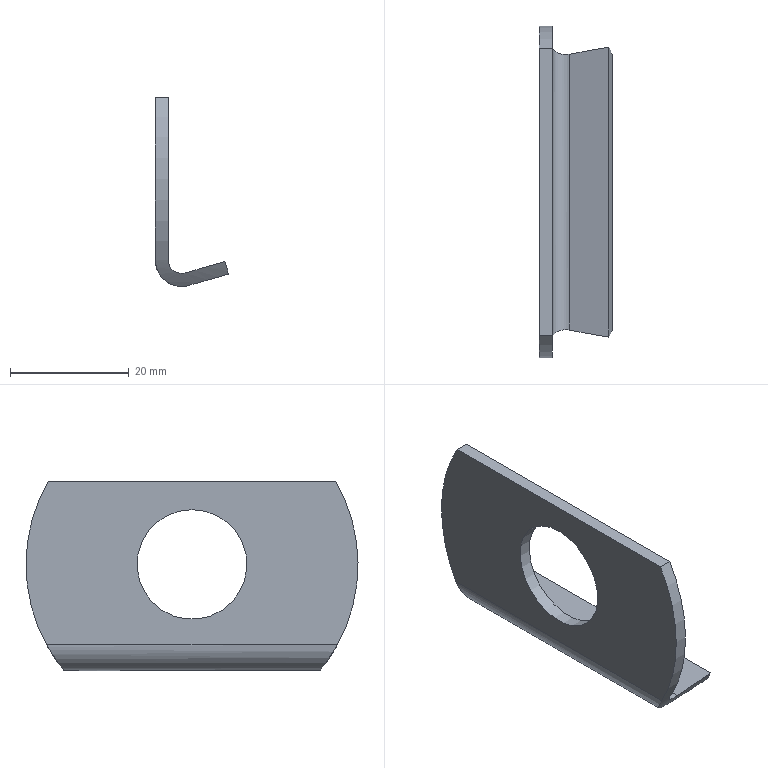Part | NX | features DATUM_CSYS 3, EXTRUDE 2, SKETCH 2, HOLE PACKAGE 1, SIMPLE HOLE 1 | 1 solid | 11 faces | box 12.342 x 56 x 31.883 mm | volume 3985 mm3 | plane 6 | cylinder 5 | commonest cylinder face diameters 56 x2 4.4 x1 8.8 x1 18.5 x1
STEP:
#1=CARTESIAN_POINT('',(2.2,24.249,33.325));
#2=VERTEX_POINT('',#1);
#3=CARTESIAN_POINT('',(0.,24.249,33.325));
#4=VERTEX_POINT('',#3);
#5=CARTESIAN_POINT('',(28.,24.249,33.325));
#6=DIRECTION('',(-1.,0.,0.));
#7=VECTOR('',#6,1000.);
#8=LINE('',#5,#7);
#9=EDGE_CURVE('',#2,#4,#8,.T.);
#10=ORIENTED_EDGE('',*,*,#9,.F.);
#11=CARTESIAN_POINT('',(2.2,24.538,5.839));
#12=VERTEX_POINT('',#11);
#13=CARTESIAN_POINT('',(2.2,0.,19.325));
#14=DIRECTION('',(-1.,0.,0.));
#15=DIRECTION('',(0.,0.,1.));
#16=AXIS2_PLACEMENT_3D('',#13,#14,#15);
#17=CIRCLE('',#16,28.);
#18=EDGE_CURVE('',#12,#2,#17,.F.);
#19=ORIENTED_EDGE('',*,*,#18,.F.);
#20=CARTESIAN_POINT('',(5.006,23.251,3.724));
#21=VERTEX_POINT('',#20);
#22=CARTESIAN_POINT('',(5.006,23.251,3.724));
#23=CARTESIAN_POINT('',(4.311,23.117,3.525));
#24=CARTESIAN_POINT('',(2.736,23.405,3.93));
#25=CARTESIAN_POINT('',(2.2,24.185,5.196));
#26=CARTESIAN_POINT('',(2.2,24.538,5.839));
#27=B_SPLINE_CURVE_WITH_KNOTS('',3,(#22,#23,#24,#25,#26),.UNSPECIFIED.,.F.,.F.,(4,1,4),(0.,0.002176,0.004352),.UNSPECIFIED.);
#28=EDGE_CURVE('',#21,#12,#27,.T.);
#29=ORIENTED_EDGE('',*,*,#28,.F.);
#30=CARTESIAN_POINT('',(11.735,24.436,5.654));
#31=VERTEX_POINT('',#30);
#32=CARTESIAN_POINT('',(59.413,0.,19.325));
#33=DIRECTION('',(0.2756,0.,-0.9613));
#34=DIRECTION('',(-0.9613,0.,-0.2756));
#35=AXIS2_PLACEMENT_3D('',#32,#33,#34);
#36=ELLIPSE('',#35,101.583,28.);
#37=EDGE_CURVE('',#31,#21,#36,.F.);
#38=ORIENTED_EDGE('',*,*,#37,.F.);
#39=CARTESIAN_POINT('',(12.342,23.126,3.539));
#40=VERTEX_POINT('',#39);
#41=CARTESIAN_POINT('',(7.815,0.,19.325));
#42=DIRECTION('',(0.9613,0.,0.2756));
#43=DIRECTION('',(-0.2756,0.,0.9613));
#44=AXIS2_PLACEMENT_3D('',#41,#42,#43);
#45=ELLIPSE('',#44,29.128,28.);
#46=EDGE_CURVE('',#40,#31,#45,.T.);
#47=ORIENTED_EDGE('',*,*,#46,.F.);
#48=CARTESIAN_POINT('',(5.613,21.683,1.609));
#49=VERTEX_POINT('',#48);
#50=CARTESIAN_POINT('',(67.394,0.,19.325));
#51=DIRECTION('',(0.2756,0.,-0.9613));
#52=DIRECTION('',(-0.9613,0.,-0.2756));
#53=AXIS2_PLACEMENT_3D('',#50,#51,#52);
#54=ELLIPSE('',#53,101.583,28.);
#55=EDGE_CURVE('',#40,#49,#54,.F.);
#56=ORIENTED_EDGE('',*,*,#55,.T.);
#57=CARTESIAN_POINT('',(0.,24.538,5.839));
#58=VERTEX_POINT('',#57);
#59=CARTESIAN_POINT('',(5.613,21.683,1.609));
#60=CARTESIAN_POINT('',(4.913,21.519,1.409));
#61=CARTESIAN_POINT('',(3.366,21.488,1.37));
#62=CARTESIAN_POINT('',(1.453,22.303,2.369));
#63=CARTESIAN_POINT('',(0.284,23.425,3.939));
#64=CARTESIAN_POINT('',(0.,24.18,5.187));
#65=CARTESIAN_POINT('',(0.,24.538,5.839));
#66=B_SPLINE_CURVE_WITH_KNOTS('',3,(#59,#60,#61,#62,#63,#64,#65),.UNSPECIFIED.,.F.,.F.,(4,1,1,1,4),(0.,0.002209,0.004418,0.006627,0.008836),.UNSPECIFIED.);
#67=EDGE_CURVE('',#49,#58,#66,.T.);
#68=ORIENTED_EDGE('',*,*,#67,.T.);
#69=CARTESIAN_POINT('',(0.,0.,19.325));
#70=DIRECTION('',(1.,0.,0.));
#71=DIRECTION('',(0.,1.,0.));
#72=AXIS2_PLACEMENT_3D('',#69,#70,#71);
#73=CIRCLE('',#72,28.);
#74=EDGE_CURVE('',#58,#4,#73,.T.);
#75=ORIENTED_EDGE('',*,*,#74,.T.);
#76=EDGE_LOOP('',(#10,#19,#29,#38,#47,#56,#68,#75));
#77=FACE_BOUND('',#76,.T.);
#78=CARTESIAN_POINT('',(28.,0.,19.325));
#79=DIRECTION('',(-1.,0.,0.));
#80=DIRECTION('',(0.,0.,1.));
#81=AXIS2_PLACEMENT_3D('',#78,#79,#80);
#82=CYLINDRICAL_SURFACE('',#81,28.);
#83=ADVANCED_FACE('',(#77),#82,.T.);
#84=CARTESIAN_POINT('',(11.735,-24.436,5.654));
#85=VERTEX_POINT('',#84);
#86=CARTESIAN_POINT('',(11.735,28.,5.654));
#87=DIRECTION('',(0.,1.,0.));
#88=VECTOR('',#87,1000.);
#89=LINE('',#86,#88);
#90=EDGE_CURVE('',#31,#85,#89,.F.);
#91=ORIENTED_EDGE('',*,*,#90,.T.);
#92=CARTESIAN_POINT('',(12.342,-23.126,3.539));
#93=VERTEX_POINT('',#92);
#94=CARTESIAN_POINT('',(7.815,0.,19.325));
#95=DIRECTION('',(0.9613,0.,0.2756));
#96=DIRECTION('',(-0.2756,0.,0.9613));
#97=AXIS2_PLACEMENT_3D('',#94,#95,#96);
#98=ELLIPSE('',#97,29.128,28.);
#99=EDGE_CURVE('',#85,#93,#98,.T.);
#100=ORIENTED_EDGE('',*,*,#99,.T.);
#101=CARTESIAN_POINT('',(12.342,28.,3.539));
#102=DIRECTION('',(0.,-1.,0.));
#103=VECTOR('',#102,1000.);
#104=LINE('',#101,#103);
#105=EDGE_CURVE('',#40,#93,#104,.T.);
#106=ORIENTED_EDGE('',*,*,#105,.F.);
#107=ORIENTED_EDGE('',*,*,#46,.T.);
#108=EDGE_LOOP('',(#91,#100,#106,#107));
#109=FACE_BOUND('',#108,.T.);
#110=CARTESIAN_POINT('',(12.342,28.,3.539));
#111=DIRECTION('',(0.9613,0.,0.2756));
#112=DIRECTION('',(0.,-1.,0.));
#113=AXIS2_PLACEMENT_3D('',#110,#111,#112);
#114=PLANE('',#113);
#115=ADVANCED_FACE('',(#109),#114,.T.);
#116=CARTESIAN_POINT('',(0.,-24.249,33.325));
#117=VERTEX_POINT('',#116);
#118=CARTESIAN_POINT('',(0.,28.,33.325));
#119=DIRECTION('',(0.,-1.,0.));
#120=VECTOR('',#119,1000.);
#121=LINE('',#118,#120);
#122=EDGE_CURVE('',#4,#117,#121,.T.);
#123=ORIENTED_EDGE('',*,*,#122,.T.);
#124=CARTESIAN_POINT('',(2.2,-24.249,33.325));
#125=VERTEX_POINT('',#124);
#126=CARTESIAN_POINT('',(28.,-24.249,33.325));
#127=DIRECTION('',(-1.,0.,0.));
#128=VECTOR('',#127,1000.);
#129=LINE('',#126,#128);
#130=EDGE_CURVE('',#117,#125,#129,.F.);
#131=ORIENTED_EDGE('',*,*,#130,.T.);
#132=CARTESIAN_POINT('',(2.2,28.,33.325));
#133=DIRECTION('',(0.,1.,0.));
#134=VECTOR('',#133,1000.);
#135=LINE('',#132,#134);
#136=EDGE_CURVE('',#2,#125,#135,.F.);
#137=ORIENTED_EDGE('',*,*,#136,.F.);
#138=ORIENTED_EDGE('',*,*,#9,.T.);
#139=EDGE_LOOP('',(#123,#131,#137,#138));
#140=FACE_BOUND('',#139,.T.);
#141=CARTESIAN_POINT('',(0.,28.,33.325));
#142=DIRECTION('',(0.,0.,-1.));
#143=DIRECTION('',(0.,-1.,0.));
#144=AXIS2_PLACEMENT_3D('',#141,#142,#143);
#145=PLANE('',#144);
#146=ADVANCED_FACE('',(#140),#145,.F.);
#147=CARTESIAN_POINT('',(2.2,0.,28.575));
#148=VERTEX_POINT('',#147);
#149=CARTESIAN_POINT('',(2.2,0.,19.325));
#150=DIRECTION('',(-1.,0.,0.));
#151=DIRECTION('',(0.,0.,1.));
#152=AXIS2_PLACEMENT_3D('',#149,#150,#151);
#153=CIRCLE('',#152,9.25);
#154=EDGE_CURVE('',#148,#148,#153,.T.);
#155=ORIENTED_EDGE('',*,*,#154,.T.);
#156=EDGE_LOOP('',(#155));
#157=FACE_BOUND('',#156,.T.);
#158=ORIENTED_EDGE('',*,*,#136,.T.);
#159=CARTESIAN_POINT('',(2.2,-24.538,5.839));
#160=VERTEX_POINT('',#159);
#161=CARTESIAN_POINT('',(2.2,0.,19.325));
#162=DIRECTION('',(-1.,0.,0.));
#163=DIRECTION('',(0.,0.,1.));
#164=AXIS2_PLACEMENT_3D('',#161,#162,#163);
#165=CIRCLE('',#164,28.);
#166=EDGE_CURVE('',#125,#160,#165,.F.);
#167=ORIENTED_EDGE('',*,*,#166,.T.);
#168=CARTESIAN_POINT('',(2.2,28.,5.839));
#169=DIRECTION('',(0.,1.,0.));
#170=VECTOR('',#169,1000.);
#171=LINE('',#168,#170);
#172=EDGE_CURVE('',#12,#160,#171,.F.);
#173=ORIENTED_EDGE('',*,*,#172,.F.);
#174=ORIENTED_EDGE('',*,*,#18,.T.);
#175=EDGE_LOOP('',(#158,#167,#173,#174));
#176=FACE_BOUND('',#175,.T.);
#177=CARTESIAN_POINT('',(2.2,28.,33.325));
#178=DIRECTION('',(-1.,0.,0.));
#179=DIRECTION('',(0.,0.,1.));
#180=AXIS2_PLACEMENT_3D('',#177,#178,#179);
#181=PLANE('',#180);
#182=ADVANCED_FACE('',(#157,#176),#181,.F.);
#183=CARTESIAN_POINT('',(5.006,-23.251,3.724));
#184=VERTEX_POINT('',#183);
#185=CARTESIAN_POINT('',(5.006,28.,3.724));
#186=DIRECTION('',(0.,-1.,0.));
#187=VECTOR('',#186,1000.);
#188=LINE('',#185,#187);
#189=EDGE_CURVE('',#21,#184,#188,.T.);
#190=ORIENTED_EDGE('',*,*,#189,.F.);
#191=ORIENTED_EDGE('',*,*,#28,.T.);
#192=ORIENTED_EDGE('',*,*,#172,.T.);
#193=CARTESIAN_POINT('',(2.2,-24.538,5.839));
#194=CARTESIAN_POINT('',(2.2,-24.184,5.195));
#195=CARTESIAN_POINT('',(2.733,-23.408,3.934));
#196=CARTESIAN_POINT('',(4.309,-23.117,3.524));
#197=CARTESIAN_POINT('',(5.006,-23.251,3.724));
#198=B_SPLINE_CURVE_WITH_KNOTS('',3,(#193,#194,#195,#196,#197),.UNSPECIFIED.,.F.,.F.,(4,1,4),(0.,0.002162,0.004324),.UNSPECIFIED.);
#199=EDGE_CURVE('',#160,#184,#198,.T.);
#200=ORIENTED_EDGE('',*,*,#199,.T.);
#201=EDGE_LOOP('',(#190,#191,#192,#200));
#202=FACE_BOUND('',#201,.T.);
#203=CARTESIAN_POINT('',(4.4,28.,5.839));
#204=DIRECTION('',(0.,-1.,0.));
#205=DIRECTION('',(0.,0.,-1.));
#206=AXIS2_PLACEMENT_3D('',#203,#204,#205);
#207=CYLINDRICAL_SURFACE('',#206,2.2);
#208=ADVANCED_FACE('',(#202),#207,.F.);
#209=ORIENTED_EDGE('',*,*,#189,.T.);
#210=CARTESIAN_POINT('',(59.413,0.,19.325));
#211=DIRECTION('',(0.2756,0.,-0.9613));
#212=DIRECTION('',(-0.9613,0.,-0.2756));
#213=AXIS2_PLACEMENT_3D('',#210,#211,#212);
#214=ELLIPSE('',#213,101.583,28.);
#215=EDGE_CURVE('',#184,#85,#214,.F.);
#216=ORIENTED_EDGE('',*,*,#215,.T.);
#217=ORIENTED_EDGE('',*,*,#90,.F.);
#218=ORIENTED_EDGE('',*,*,#37,.T.);
#219=EDGE_LOOP('',(#209,#216,#217,#218));
#220=FACE_BOUND('',#219,.T.);
#221=CARTESIAN_POINT('',(5.006,28.,3.724));
#222=DIRECTION('',(0.2756,0.,-0.9613));
#223=DIRECTION('',(-0.9613,0.,-0.2756));
#224=AXIS2_PLACEMENT_3D('',#221,#222,#223);
#225=PLANE('',#224);
#226=ADVANCED_FACE('',(#220),#225,.F.);
#227=CARTESIAN_POINT('',(0.,0.,28.575));
#228=VERTEX_POINT('',#227);
#229=CARTESIAN_POINT('',(0.,0.,19.325));
#230=DIRECTION('',(-1.,0.,0.));
#231=DIRECTION('',(0.,0.,1.));
#232=AXIS2_PLACEMENT_3D('',#229,#230,#231);
#233=CIRCLE('',#232,9.25);
#234=EDGE_CURVE('',#228,#228,#233,.T.);
#235=ORIENTED_EDGE('',*,*,#234,.F.);
#236=EDGE_LOOP('',(#235));
#237=FACE_BOUND('',#236,.T.);
#238=CARTESIAN_POINT('',(0.,-24.538,5.839));
#239=VERTEX_POINT('',#238);
#240=CARTESIAN_POINT('',(0.,0.,19.325));
#241=DIRECTION('',(1.,0.,0.));
#242=DIRECTION('',(0.,1.,0.));
#243=AXIS2_PLACEMENT_3D('',#240,#241,#242);
#244=CIRCLE('',#243,28.);
#245=EDGE_CURVE('',#117,#239,#244,.T.);
#246=ORIENTED_EDGE('',*,*,#245,.F.);
#247=ORIENTED_EDGE('',*,*,#122,.F.);
#248=ORIENTED_EDGE('',*,*,#74,.F.);
#249=CARTESIAN_POINT('',(0.,28.,5.839));
#250=DIRECTION('',(0.,-1.,0.));
#251=VECTOR('',#250,1000.);
#252=LINE('',#249,#251);
#253=EDGE_CURVE('',#58,#239,#252,.T.);
#254=ORIENTED_EDGE('',*,*,#253,.T.);
#255=EDGE_LOOP('',(#246,#247,#248,#254));
#256=FACE_BOUND('',#255,.T.);
#257=CARTESIAN_POINT('',(0.,28.,33.325));
#258=DIRECTION('',(-1.,0.,0.));
#259=DIRECTION('',(0.,0.,1.));
#260=AXIS2_PLACEMENT_3D('',#257,#258,#259);
#261=PLANE('',#260);
#262=ADVANCED_FACE('',(#237,#256),#261,.T.);
#263=ORIENTED_EDGE('',*,*,#67,.F.);
#264=CARTESIAN_POINT('',(5.613,-21.683,1.609));
#265=VERTEX_POINT('',#264);
#266=CARTESIAN_POINT('',(5.613,28.,1.609));
#267=DIRECTION('',(0.,-1.,0.));
#268=VECTOR('',#267,1000.);
#269=LINE('',#266,#268);
#270=EDGE_CURVE('',#49,#265,#269,.T.);
#271=ORIENTED_EDGE('',*,*,#270,.T.);
#272=CARTESIAN_POINT('',(0.,-24.538,5.839));
#273=CARTESIAN_POINT('',(0.,-24.18,5.186));
#274=CARTESIAN_POINT('',(0.2822,-23.428,3.944));
#275=CARTESIAN_POINT('',(1.45,-22.306,2.372));
#276=CARTESIAN_POINT('',(3.355,-21.489,1.372));
#277=CARTESIAN_POINT('',(4.911,-21.519,1.408));
#278=CARTESIAN_POINT('',(5.613,-21.683,1.609));
#279=B_SPLINE_CURVE_WITH_KNOTS('',3,(#272,#273,#274,#275,#276,#277,#278),.UNSPECIFIED.,.F.,.F.,(4,1,1,1,4),(0.,0.002192,0.004384,0.006577,0.008769),.UNSPECIFIED.);
#280=EDGE_CURVE('',#239,#265,#279,.T.);
#281=ORIENTED_EDGE('',*,*,#280,.F.);
#282=ORIENTED_EDGE('',*,*,#253,.F.);
#283=EDGE_LOOP('',(#263,#271,#281,#282));
#284=FACE_BOUND('',#283,.T.);
#285=CARTESIAN_POINT('',(4.4,28.,5.839));
#286=DIRECTION('',(0.,-1.,0.));
#287=DIRECTION('',(0.,0.,-1.));
#288=AXIS2_PLACEMENT_3D('',#285,#286,#287);
#289=CYLINDRICAL_SURFACE('',#288,4.4);
#290=ADVANCED_FACE('',(#284),#289,.T.);
#291=CARTESIAN_POINT('',(67.394,0.,19.325));
#292=DIRECTION('',(0.2756,0.,-0.9613));
#293=DIRECTION('',(-0.9613,0.,-0.2756));
#294=AXIS2_PLACEMENT_3D('',#291,#292,#293);
#295=ELLIPSE('',#294,101.583,28.);
#296=EDGE_CURVE('',#265,#93,#295,.F.);
#297=ORIENTED_EDGE('',*,*,#296,.F.);
#298=ORIENTED_EDGE('',*,*,#270,.F.);
#299=ORIENTED_EDGE('',*,*,#55,.F.);
#300=ORIENTED_EDGE('',*,*,#105,.T.);
#301=EDGE_LOOP('',(#297,#298,#299,#300));
#302=FACE_BOUND('',#301,.T.);
#303=CARTESIAN_POINT('',(5.613,28.,1.609));
#304=DIRECTION('',(0.2756,0.,-0.9613));
#305=DIRECTION('',(-0.9613,0.,-0.2756));
#306=AXIS2_PLACEMENT_3D('',#303,#304,#305);
#307=PLANE('',#306);
#308=ADVANCED_FACE('',(#302),#307,.T.);
#309=ORIENTED_EDGE('',*,*,#199,.F.);
#310=ORIENTED_EDGE('',*,*,#166,.F.);
#311=ORIENTED_EDGE('',*,*,#130,.F.);
#312=ORIENTED_EDGE('',*,*,#245,.T.);
#313=ORIENTED_EDGE('',*,*,#280,.T.);
#314=ORIENTED_EDGE('',*,*,#296,.T.);
#315=ORIENTED_EDGE('',*,*,#99,.F.);
#316=ORIENTED_EDGE('',*,*,#215,.F.);
#317=EDGE_LOOP('',(#309,#310,#311,#312,#313,#314,#315,#316));
#318=FACE_BOUND('',#317,.T.);
#319=CARTESIAN_POINT('',(28.,0.,19.325));
#320=DIRECTION('',(-1.,0.,0.));
#321=DIRECTION('',(0.,0.,1.));
#322=AXIS2_PLACEMENT_3D('',#319,#320,#321);
#323=CYLINDRICAL_SURFACE('',#322,28.);
#324=ADVANCED_FACE('',(#318),#323,.T.);
#325=ORIENTED_EDGE('',*,*,#234,.T.);
#326=EDGE_LOOP('',(#325));
#327=FACE_BOUND('',#326,.T.);
#328=ORIENTED_EDGE('',*,*,#154,.F.);
#329=EDGE_LOOP('',(#328));
#330=FACE_BOUND('',#329,.T.);
#331=CARTESIAN_POINT('',(2.2,0.,19.325));
#332=DIRECTION('',(-1.,0.,0.));
#333=DIRECTION('',(0.,0.,1.));
#334=AXIS2_PLACEMENT_3D('',#331,#332,#333);
#335=CYLINDRICAL_SURFACE('',#334,9.25);
#336=ADVANCED_FACE('',(#327,#330),#335,.F.);
#337=CLOSED_SHELL('',(#83,#115,#146,#182,#208,#226,#262,#290,#308,#324,#336));
#338=MANIFOLD_SOLID_BREP('',#337);
#339=(LENGTH_UNIT()NAMED_UNIT(*)SI_UNIT(.MILLI.,.METRE.));
#340=UNCERTAINTY_MEASURE_WITH_UNIT(LENGTH_MEASURE(0.0508),#339,'','');
#341=(NAMED_UNIT(*)PLANE_ANGLE_UNIT()SI_UNIT($,.RADIAN.));
#342=(NAMED_UNIT(*)SI_UNIT($,.STERADIAN.)SOLID_ANGLE_UNIT());
#343=(GEOMETRIC_REPRESENTATION_CONTEXT(3)GLOBAL_UNCERTAINTY_ASSIGNED_CONTEXT((#340))GLOBAL_UNIT_ASSIGNED_CONTEXT((#339,#341,#342))REPRESENTATION_CONTEXT('',''));
#344=ADVANCED_BREP_SHAPE_REPRESENTATION('',(#338),#343);